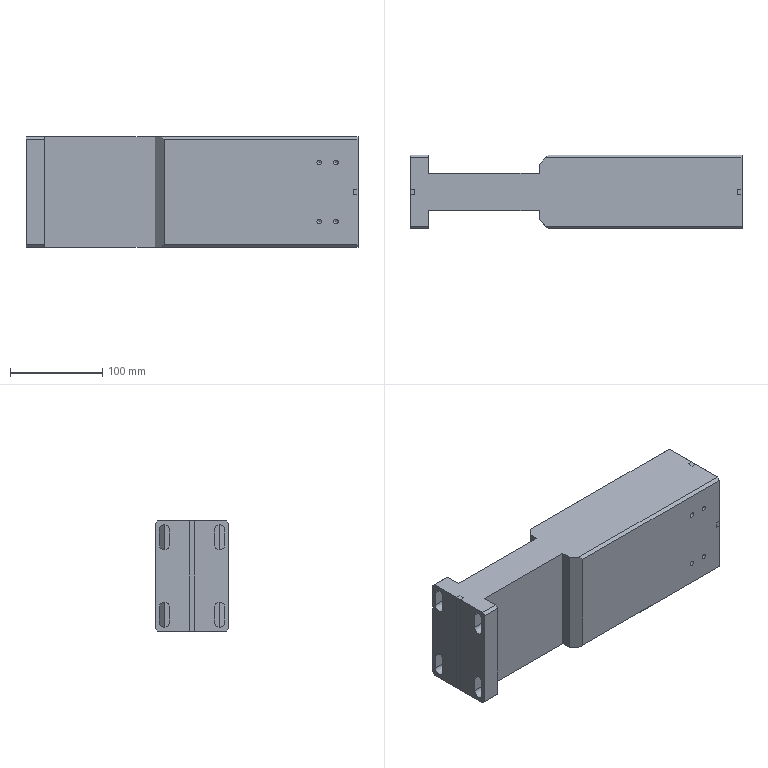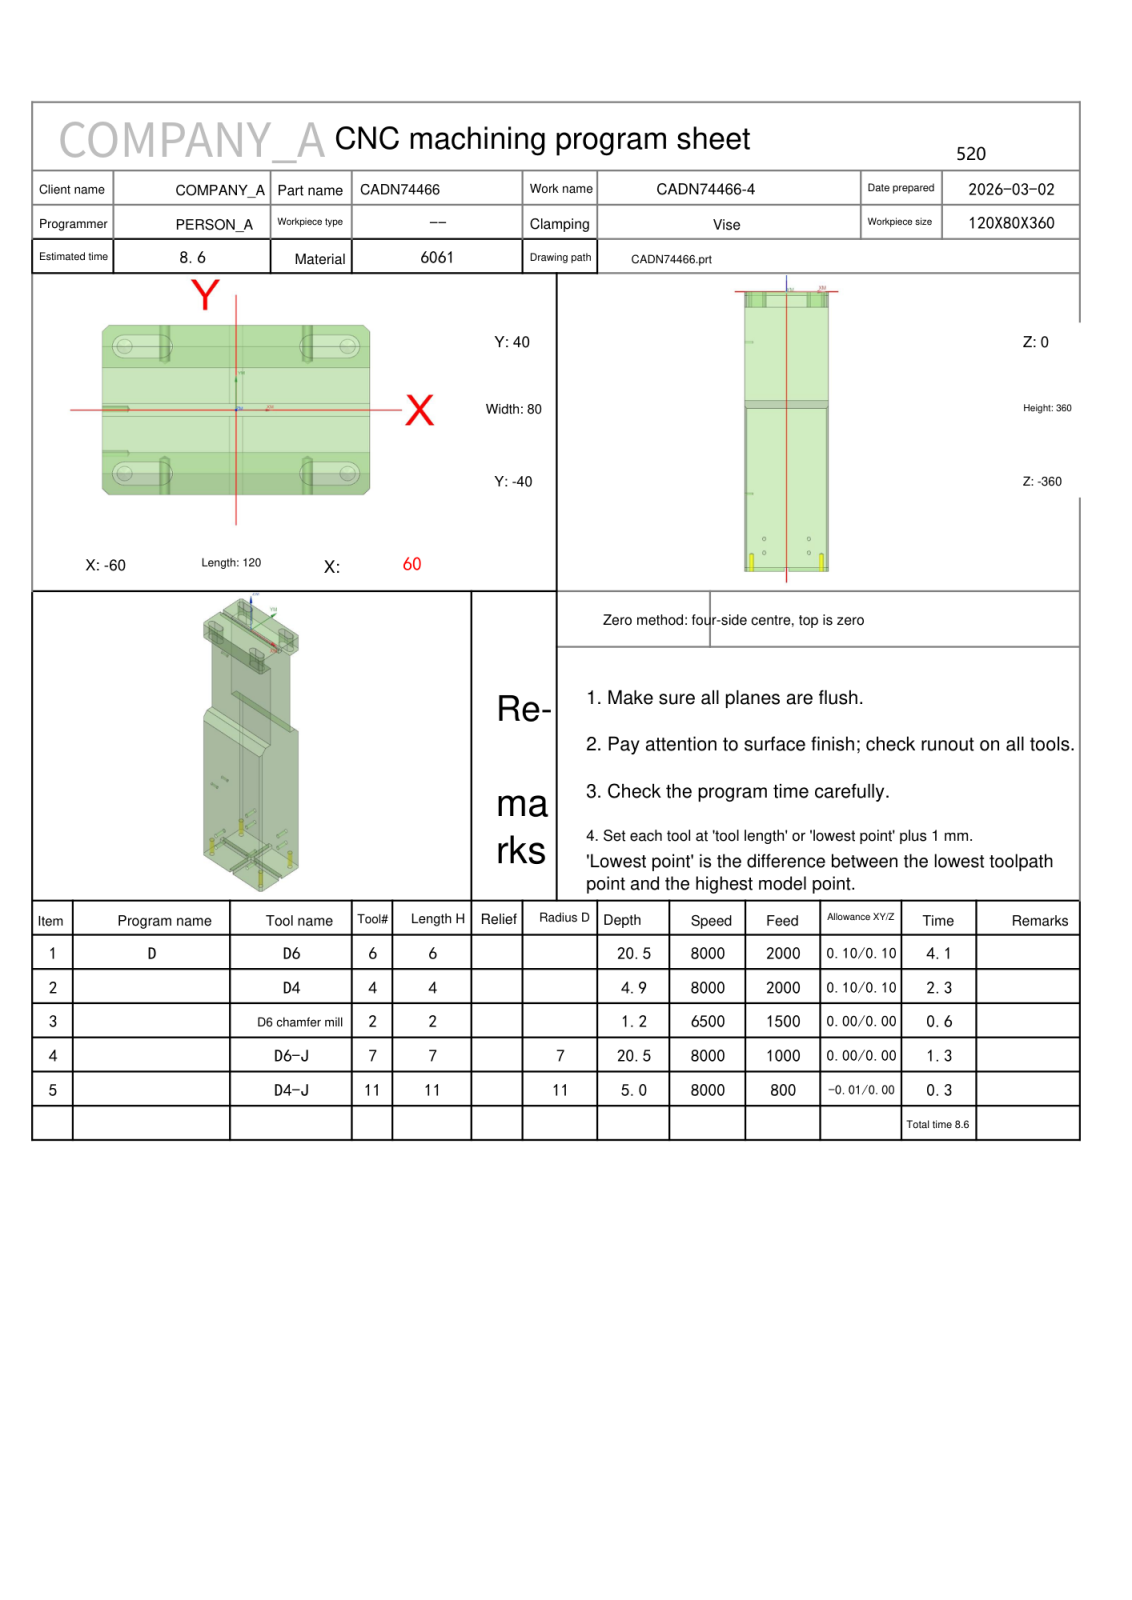NC program | NX | posted by the shop | part box 360 x 80 x 120 mm
Whole program, first 1424 of 1794 lines:
%
O0001
(Machine time: 9.60 MIN)
(===Total Tool:5===)
(T6=D6      D=6.   R=0.   D-  H06 Z=-20.5 )
(T4=D4      D=4.   R=0.   D-  H04 Z=-4.9  )
(T2=D6 chamfer mill   D=6.   R=0.   D-  H02 Z=-1.2  )
(T7=D6-J    D=6.   R=0.   D7  H07 Z=-20.5 )
(T11=D4-J   D=4.   R=0.   D11 H11 Z=-5.   )
G80 G90 G17 G49 G40
G91 G28 Z0
M01
N1 T06 M06
(D6  D=6. R=0. H=06 ce=0.10 di=0.10)
G00 G90 G54 X-38.502 Y-27.6 M03 S8000
G43 H06 Z50.
M08
Z1.
G01 X-50.381 Z.377 F2000.
X-51.324 Y-27.962 Z.325
X-52.038 Y-28.676 Z.272
X-52.4 Y-29.619 Z.219
Y-30.381 Z.179
X-52.038 Y-31.324 Z.126
X-51.324 Y-32.038 Z.073
X-50.381 Y-32.4 Z.02
X-50. Z0.0
X-34. Z-.166
G03 X-31.6 Y-30. Z-.205 I0.0 J2.4
X-34. Y-27.6 Z-.244 I-2.4 J0.0
G01 X-50. Z-.41
G03 X-52.4 Y-30. Z-.449 I0.0 J-2.4
X-50. Y-32.4 Z-.488 I2.4 J0.0
G01 X-34. Z-.654
G03 X-31.6 Y-30. Z-.693 I0.0 J2.4
X-34. Y-27.6 Z-.732 I-2.4 J0.0
G01 X-50. Z-.898
G03 X-52.4 Y-30. Z-.937 I0.0 J-2.4
X-50. Y-32.4 Z-.976 I2.4 J0.0
G01 X-34. Z-1.142
G03 X-31.6 Y-30. Z-1.181 I0.0 J2.4
X-34. Y-27.6 Z-1.22 I-2.4 J0.0
G01 X-50. Z-1.386
G03 X-52.4 Y-30. Z-1.425 I0.0 J-2.4
X-50. Y-32.4 Z-1.464 I2.4 J0.0
G01 X-34. Z-1.63
G03 X-31.6 Y-30. Z-1.669 I0.0 J2.4
X-34. Y-27.6 Z-1.708 I-2.4 J0.0
G01 X-50. Z-1.874
G03 X-52.4 Y-30. Z-1.913 I0.0 J-2.4
X-50. Y-32.4 Z-1.952 I2.4 J0.0
G01 X-34. Z-2.118
G03 X-31.6 Y-30. Z-2.157 I0.0 J2.4
X-34. Y-27.6 Z-2.196 I-2.4 J0.0
G01 X-50. Z-2.362
G03 X-52.4 Y-30. Z-2.401 I0.0 J-2.4
X-50. Y-32.4 Z-2.44 I2.4 J0.0
G01 X-34. Z-2.606
G03 X-31.6 Y-30. Z-2.645 I0.0 J2.4
X-34. Y-27.6 Z-2.685 I-2.4 J0.0
G01 X-50. Z-2.85
G03 X-52.4 Y-30. Z-2.889 I0.0 J-2.4
X-50. Y-32.4 Z-2.929 I2.4 J0.0
G01 X-34. Z-3.094
G03 X-31.6 Y-30. Z-3.134 I0.0 J2.4
X-34. Y-27.6 Z-3.173 I-2.4 J0.0
G01 X-50. Z-3.338
G03 X-52.4 Y-30. Z-3.378 I0.0 J-2.4
X-50. Y-32.4 Z-3.417 I2.4 J0.0
G01 X-34. Z-3.583
G03 X-31.6 Y-30. Z-3.622 I0.0 J2.4
X-34. Y-27.6 Z-3.661 I-2.4 J0.0
G01 X-50. Z-3.827
G03 X-52.4 Y-30. Z-3.866 I0.0 J-2.4
X-50. Y-32.4 Z-3.905 I2.4 J0.0
G01 X-34. Z-4.071
G03 X-31.6 Y-30. Z-4.11 I0.0 J2.4
X-34. Y-27.6 Z-4.149 I-2.4 J0.0
G01 X-50. Z-4.315
G03 X-52.4 Y-30. Z-4.354 I0.0 J-2.4
X-50. Y-32.4 Z-4.393 I2.4 J0.0
G01 X-34. Z-4.559
G03 X-31.6 Y-30. Z-4.598 I0.0 J2.4
X-34. Y-27.6 Z-4.637 I-2.4 J0.0
G01 X-50. Z-4.803
G03 X-52.4 Y-30. Z-4.842 I0.0 J-2.4
X-50. Y-32.4 Z-4.881 I2.4 J0.0
G01 X-34. Z-5.047
G03 X-31.6 Y-30. Z-5.086 I0.0 J2.4
X-34. Y-27.6 Z-5.125 I-2.4 J0.0
G01 X-50. Z-5.291
G03 X-52.4 Y-30. Z-5.33 I0.0 J-2.4
X-50. Y-32.4 Z-5.369 I2.4 J0.0
G01 X-34. Z-5.535
G03 X-31.6 Y-30. Z-5.574 I0.0 J2.4
X-34. Y-27.6 Z-5.613 I-2.4 J0.0
G01 X-50. Z-5.779
G03 X-52.4 Y-30. Z-5.818 I0.0 J-2.4
X-50. Y-32.4 Z-5.857 I2.4 J0.0
G01 X-34. Z-6.023
G03 X-31.6 Y-30. Z-6.062 I0.0 J2.4
X-34. Y-27.6 Z-6.101 I-2.4 J0.0
G01 X-50. Z-6.267
G03 X-52.4 Y-30. Z-6.306 I0.0 J-2.4
X-50. Y-32.4 Z-6.345 I2.4 J0.0
G01 X-34. Z-6.511
G03 X-31.6 Y-30. Z-6.55 I0.0 J2.4
X-34. Y-27.6 Z-6.589 I-2.4 J0.0
G01 X-50. Z-6.755
G03 X-52.4 Y-30. Z-6.794 I0.0 J-2.4
X-50. Y-32.4 Z-6.833 I2.4 J0.0
G01 X-34. Z-6.999
G03 X-31.6 Y-30. Z-7.038 I0.0 J2.4
X-34. Y-27.6 Z-7.077 I-2.4 J0.0
G01 X-50. Z-7.243
G03 X-52.4 Y-30. Z-7.282 I0.0 J-2.4
X-50. Y-32.4 Z-7.321 I2.4 J0.0
G01 X-34. Z-7.487
G03 X-31.6 Y-30. Z-7.526 I0.0 J2.4
X-34. Y-27.6 Z-7.565 I-2.4 J0.0
G01 X-50. Z-7.731
G03 X-52.4 Y-30. Z-7.77 I0.0 J-2.4
X-50. Y-32.4 Z-7.81 I2.4 J0.0
G01 X-34. Z-7.975
G03 X-31.6 Y-30. Z-8.014 I0.0 J2.4
X-34. Y-27.6 Z-8.054 I-2.4 J0.0
G01 X-50. Z-8.219
G03 X-52.4 Y-30. Z-8.259 I0.0 J-2.4
X-50. Y-32.4 Z-8.298 I2.4 J0.0
G01 X-34. Z-8.463
G03 X-31.6 Y-30. Z-8.503 I0.0 J2.4
X-34. Y-27.6 Z-8.542 I-2.4 J0.0
G01 X-50. Z-8.708
G03 X-52.4 Y-30. Z-8.747 I0.0 J-2.4
X-50. Y-32.4 Z-8.786 I2.4 J0.0
G01 X-34. Z-8.952
G03 X-31.6 Y-30. Z-8.991 I0.0 J2.4
X-34. Y-27.6 Z-9.03 I-2.4 J0.0
G01 X-50. Z-9.196
G03 X-52.4 Y-30. Z-9.235 I0.0 J-2.4
X-50. Y-32.4 Z-9.274 I2.4 J0.0
G01 X-34. Z-9.44
G03 X-31.6 Y-30. Z-9.479 I0.0 J2.4
X-34. Y-27.6 Z-9.518 I-2.4 J0.0
G01 X-50. Z-9.684
G03 X-52.4 Y-30. Z-9.723 I0.0 J-2.4
X-50. Y-32.4 Z-9.762 I2.4 J0.0
G01 X-34. Z-9.928
G03 X-31.6 Y-30. Z-9.967 I0.0 J2.4
X-34. Y-27.6 Z-10.006 I-2.4 J0.0
G01 X-50. Z-10.172
G03 X-52.4 Y-30. Z-10.211 I0.0 J-2.4
X-50. Y-32.4 Z-10.25 I2.4 J0.0
G01 X-34. Z-10.416
G03 X-31.6 Y-30. Z-10.455 I0.0 J2.4
X-34. Y-27.6 Z-10.494 I-2.4 J0.0
G01 X-50. Z-10.66
G03 X-52.4 Y-30. Z-10.699 I0.0 J-2.4
X-50. Y-32.4 Z-10.738 I2.4 J0.0
G01 X-34. Z-10.904
G03 X-31.6 Y-30. Z-10.943 I0.0 J2.4
X-34. Y-27.6 Z-10.982 I-2.4 J0.0
G01 X-50. Z-11.148
G03 X-52.4 Y-30. Z-11.187 I0.0 J-2.4
X-50. Y-32.4 Z-11.226 I2.4 J0.0
G01 X-34. Z-11.392
G03 X-31.6 Y-30. Z-11.431 I0.0 J2.4
X-34. Y-27.6 Z-11.47 I-2.4 J0.0
G01 X-50. Z-11.636
G03 X-52.4 Y-30. Z-11.675 I0.0 J-2.4
X-50. Y-32.4 Z-11.714 I2.4 J0.0
G01 X-34. Z-11.88
G03 X-31.6 Y-30. Z-11.919 I0.0 J2.4
X-34. Y-27.6 Z-11.958 I-2.4 J0.0
G01 X-50. Z-12.124
G03 X-52.4 Y-30. Z-12.163 I0.0 J-2.4
X-50. Y-32.4 Z-12.202 I2.4 J0.0
G01 X-34. Z-12.368
G03 X-31.6 Y-30. Z-12.407 I0.0 J2.4
X-34. Y-27.6 Z-12.446 I-2.4 J0.0
G01 X-50. Z-12.612
G03 X-52.4 Y-30. Z-12.651 I0.0 J-2.4
X-50. Y-32.4 Z-12.69 I2.4 J0.0
G01 X-34. Z-12.856
G03 X-31.6 Y-30. Z-12.895 I0.0 J2.4
X-34. Y-27.6 Z-12.935 I-2.4 J0.0
G01 X-50. Z-13.1
G03 X-52.4 Y-30. Z-13.139 I0.0 J-2.4
X-50. Y-32.4 Z-13.179 I2.4 J0.0
G01 X-34. Z-13.344
G03 X-31.6 Y-30. Z-13.384 I0.0 J2.4
X-34. Y-27.6 Z-13.423 I-2.4 J0.0
G01 X-50. Z-13.588
G03 X-52.4 Y-30. Z-13.628 I0.0 J-2.4
X-50. Y-32.4 Z-13.667 I2.4 J0.0
G01 X-34. Z-13.833
G03 X-31.6 Y-30. Z-13.872 I0.0 J2.4
X-34. Y-27.6 Z-13.911 I-2.4 J0.0
G01 X-50. Z-14.077
G03 X-52.4 Y-30. Z-14.116 I0.0 J-2.4
X-50. Y-32.4 Z-14.155 I2.4 J0.0
G01 X-34. Z-14.321
G03 X-31.6 Y-30. Z-14.36 I0.0 J2.4
X-34. Y-27.6 Z-14.399 I-2.4 J0.0
G01 X-50. Z-14.565
G03 X-52.4 Y-30. Z-14.604 I0.0 J-2.4
X-50. Y-32.4 Z-14.643 I2.4 J0.0
G01 X-34. Z-14.809
G03 X-31.6 Y-30. Z-14.848 I0.0 J2.4
X-34. Y-27.6 Z-14.887 I-2.4 J0.0
G01 X-50. Z-15.053
G03 X-52.4 Y-30. Z-15.092 I0.0 J-2.4
X-50. Y-32.4 Z-15.131 I2.4 J0.0
G01 X-34. Z-15.297
G03 X-31.6 Y-30. Z-15.336 I0.0 J2.4
X-34. Y-27.6 Z-15.375 I-2.4 J0.0
G01 X-50. Z-15.541
G03 X-52.4 Y-30. Z-15.58 I0.0 J-2.4
X-50. Y-32.4 Z-15.619 I2.4 J0.0
G01 X-34. Z-15.785
G03 X-31.6 Y-30. Z-15.824 I0.0 J2.4
X-34. Y-27.6 Z-15.863 I-2.4 J0.0
G01 X-50. Z-16.029
G03 X-52.4 Y-30. Z-16.068 I0.0 J-2.4
X-50. Y-32.4 Z-16.107 I2.4 J0.0
G01 X-34. Z-16.273
G03 X-31.6 Y-30. Z-16.312 I0.0 J2.4
X-34. Y-27.6 Z-16.351 I-2.4 J0.0
G01 X-50. Z-16.517
G03 X-52.4 Y-30. Z-16.556 I0.0 J-2.4
X-50. Y-32.4 Z-16.595 I2.4 J0.0
G01 X-34. Z-16.761
G03 X-31.6 Y-30. Z-16.8 I0.0 J2.4
X-34. Y-27.6 Z-16.839 I-2.4 J0.0
G01 X-50. Z-17.005
G03 X-52.4 Y-30. Z-17.044 I0.0 J-2.4
X-50. Y-32.4 Z-17.083 I2.4 J0.0
G01 X-34. Z-17.249
G03 X-31.6 Y-30. Z-17.288 I0.0 J2.4
X-34. Y-27.6 Z-17.327 I-2.4 J0.0
G01 X-50. Z-17.493
G03 X-52.4 Y-30. Z-17.532 I0.0 J-2.4
X-50. Y-32.4 Z-17.571 I2.4 J0.0
G01 X-34. Z-17.737
G03 X-31.6 Y-30. Z-17.776 I0.0 J2.4
X-34. Y-27.6 Z-17.815 I-2.4 J0.0
G01 X-50. Z-17.981
G03 X-52.4 Y-30. Z-18.02 I0.0 J-2.4
X-50. Y-32.4 Z-18.06 I2.4 J0.0
G01 X-34. Z-18.225
G03 X-31.6 Y-30. Z-18.264 I0.0 J2.4
X-34. Y-27.6 Z-18.304 I-2.4 J0.0
G01 X-50. Z-18.469
G03 X-52.4 Y-30. Z-18.509 I0.0 J-2.4
X-50. Y-32.4 Z-18.548 I2.4 J0.0
G01 X-34. Z-18.713
G03 X-31.6 Y-30. Z-18.753 I0.0 J2.4
X-34. Y-27.6 Z-18.792 I-2.4 J0.0
G01 X-50. Z-18.958
G03 X-52.4 Y-30. Z-18.997 I0.0 J-2.4
X-50. Y-32.4 Z-19.036 I2.4 J0.0
G01 X-34. Z-19.202
G03 X-31.6 Y-30. Z-19.241 I0.0 J2.4
X-34. Y-27.6 Z-19.28 I-2.4 J0.0
G01 X-50. Z-19.446
G03 X-52.4 Y-30. Z-19.485 I0.0 J-2.4
X-50. Y-32.4 Z-19.524 I2.4 J0.0
G01 X-34. Z-19.69
G03 X-31.6 Y-30. Z-19.729 I0.0 J2.4
X-34. Y-27.6 Z-19.768 I-2.4 J0.0
G01 X-50. Z-19.934
G03 X-52.4 Y-30. Z-19.973 I0.0 J-2.4
X-50. Y-32.4 Z-20.012 I2.4 J0.0
G01 X-34. Z-20.178
G03 X-31.6 Y-30. Z-20.217 I0.0 J2.4
X-34. Y-27.6 Z-20.256 I-2.4 J0.0
G01 X-50. Z-20.422
G03 X-52.4 Y-30. Z-20.461 I0.0 J-2.4
X-50. Y-32.4 Z-20.5 I2.4 J0.0
G01 X-34.
G03 X-31.6 Y-30. I0.0 J2.4
X-34. Y-27.6 I-2.4 J0.0
G01 X-50.
G03 X-52.4 Y-30. I0.0 J-2.4
X-50. Y-32.4 I2.4 J0.0
G01 X-49.6
Z-19.5
G00 Z50.
X-45.498 Y27.6
Z1.
G01 X-33.619 Z.377
X-32.676 Y27.962 Z.325
X-31.962 Y28.676 Z.272
X-31.6 Y29.619 Z.219
Y30.381 Z.179
X-31.962 Y31.324 Z.126
X-32.676 Y32.038 Z.073
X-33.619 Y32.4 Z.02
X-34. Z0.0
X-50. Z-.166
G03 X-52.4 Y30. Z-.205 I0.0 J-2.4
X-50. Y27.6 Z-.244 I2.4 J0.0
G01 X-34. Z-.41
G03 X-31.6 Y30. Z-.449 I0.0 J2.4
X-34. Y32.4 Z-.488 I-2.4 J0.0
G01 X-50. Z-.654
G03 X-52.4 Y30. Z-.693 I0.0 J-2.4
X-50. Y27.6 Z-.732 I2.4 J0.0
G01 X-34. Z-.898
G03 X-31.6 Y30. Z-.937 I0.0 J2.4
X-34. Y32.4 Z-.976 I-2.4 J0.0
G01 X-50. Z-1.142
G03 X-52.4 Y30. Z-1.181 I0.0 J-2.4
X-50. Y27.6 Z-1.22 I2.4 J0.0
G01 X-34. Z-1.386
G03 X-31.6 Y30. Z-1.425 I0.0 J2.4
X-34. Y32.4 Z-1.464 I-2.4 J0.0
G01 X-50. Z-1.63
G03 X-52.4 Y30. Z-1.669 I0.0 J-2.4
X-50. Y27.6 Z-1.708 I2.4 J0.0
G01 X-34. Z-1.874
G03 X-31.6 Y30. Z-1.913 I0.0 J2.4
X-34. Y32.4 Z-1.952 I-2.4 J0.0
G01 X-50. Z-2.118
G03 X-52.4 Y30. Z-2.157 I0.0 J-2.4
X-50. Y27.6 Z-2.196 I2.4 J0.0
G01 X-34. Z-2.362
G03 X-31.6 Y30. Z-2.401 I0.0 J2.4
X-34. Y32.4 Z-2.44 I-2.4 J0.0
G01 X-50. Z-2.606
G03 X-52.4 Y30. Z-2.645 I0.0 J-2.4
X-50. Y27.6 Z-2.685 I2.4 J0.0
G01 X-34. Z-2.85
G03 X-31.6 Y30. Z-2.889 I0.0 J2.4
X-34. Y32.4 Z-2.929 I-2.4 J0.0
G01 X-50. Z-3.094
G03 X-52.4 Y30. Z-3.134 I0.0 J-2.4
X-50. Y27.6 Z-3.173 I2.4 J0.0
G01 X-34. Z-3.338
G03 X-31.6 Y30. Z-3.378 I0.0 J2.4
X-34. Y32.4 Z-3.417 I-2.4 J0.0
G01 X-50. Z-3.583
G03 X-52.4 Y30. Z-3.622 I0.0 J-2.4
X-50. Y27.6 Z-3.661 I2.4 J0.0
G01 X-34. Z-3.827
G03 X-31.6 Y30. Z-3.866 I0.0 J2.4
X-34. Y32.4 Z-3.905 I-2.4 J0.0
G01 X-50. Z-4.071
G03 X-52.4 Y30. Z-4.11 I0.0 J-2.4
X-50. Y27.6 Z-4.149 I2.4 J0.0
G01 X-34. Z-4.315
G03 X-31.6 Y30. Z-4.354 I0.0 J2.4
X-34. Y32.4 Z-4.393 I-2.4 J0.0
G01 X-50. Z-4.559
G03 X-52.4 Y30. Z-4.598 I0.0 J-2.4
X-50. Y27.6 Z-4.637 I2.4 J0.0
G01 X-34. Z-4.803
G03 X-31.6 Y30. Z-4.842 I0.0 J2.4
X-34. Y32.4 Z-4.881 I-2.4 J0.0
G01 X-50. Z-5.047
G03 X-52.4 Y30. Z-5.086 I0.0 J-2.4
X-50. Y27.6 Z-5.125 I2.4 J0.0
G01 X-34. Z-5.291
G03 X-31.6 Y30. Z-5.33 I0.0 J2.4
X-34. Y32.4 Z-5.369 I-2.4 J0.0
G01 X-50. Z-5.535
G03 X-52.4 Y30. Z-5.574 I0.0 J-2.4
X-50. Y27.6 Z-5.613 I2.4 J0.0
G01 X-34. Z-5.779
G03 X-31.6 Y30. Z-5.818 I0.0 J2.4
X-34. Y32.4 Z-5.857 I-2.4 J0.0
G01 X-50. Z-6.023
G03 X-52.4 Y30. Z-6.062 I0.0 J-2.4
X-50. Y27.6 Z-6.101 I2.4 J0.0
G01 X-34. Z-6.267
G03 X-31.6 Y30. Z-6.306 I0.0 J2.4
X-34. Y32.4 Z-6.345 I-2.4 J0.0
G01 X-50. Z-6.511
G03 X-52.4 Y30. Z-6.55 I0.0 J-2.4
X-50. Y27.6 Z-6.589 I2.4 J0.0
G01 X-34. Z-6.755
G03 X-31.6 Y30. Z-6.794 I0.0 J2.4
X-34. Y32.4 Z-6.833 I-2.4 J0.0
G01 X-50. Z-6.999
G03 X-52.4 Y30. Z-7.038 I0.0 J-2.4
X-50. Y27.6 Z-7.077 I2.4 J0.0
G01 X-34. Z-7.243
G03 X-31.6 Y30. Z-7.282 I0.0 J2.4
X-34. Y32.4 Z-7.321 I-2.4 J0.0
G01 X-50. Z-7.487
G03 X-52.4 Y30. Z-7.526 I0.0 J-2.4
X-50. Y27.6 Z-7.565 I2.4 J0.0
G01 X-34. Z-7.731
G03 X-31.6 Y30. Z-7.77 I0.0 J2.4
X-34. Y32.4 Z-7.81 I-2.4 J0.0
G01 X-50. Z-7.975
G03 X-52.4 Y30. Z-8.014 I0.0 J-2.4
X-50. Y27.6 Z-8.054 I2.4 J0.0
G01 X-34. Z-8.219
G03 X-31.6 Y30. Z-8.259 I0.0 J2.4
X-34. Y32.4 Z-8.298 I-2.4 J0.0
G01 X-50. Z-8.463
G03 X-52.4 Y30. Z-8.503 I0.0 J-2.4
X-50. Y27.6 Z-8.542 I2.4 J0.0
G01 X-34. Z-8.708
G03 X-31.6 Y30. Z-8.747 I0.0 J2.4
X-34. Y32.4 Z-8.786 I-2.4 J0.0
G01 X-50. Z-8.952
G03 X-52.4 Y30. Z-8.991 I0.0 J-2.4
X-50. Y27.6 Z-9.03 I2.4 J0.0
G01 X-34. Z-9.196
G03 X-31.6 Y30. Z-9.235 I0.0 J2.4
X-34. Y32.4 Z-9.274 I-2.4 J0.0
G01 X-50. Z-9.44
G03 X-52.4 Y30. Z-9.479 I0.0 J-2.4
X-50. Y27.6 Z-9.518 I2.4 J0.0
G01 X-34. Z-9.684
G03 X-31.6 Y30. Z-9.723 I0.0 J2.4
X-34. Y32.4 Z-9.762 I-2.4 J0.0
G01 X-50. Z-9.928
G03 X-52.4 Y30. Z-9.967 I0.0 J-2.4
X-50. Y27.6 Z-10.006 I2.4 J0.0
G01 X-34. Z-10.172
G03 X-31.6 Y30. Z-10.211 I0.0 J2.4
X-34. Y32.4 Z-10.25 I-2.4 J0.0
G01 X-50. Z-10.416
G03 X-52.4 Y30. Z-10.455 I0.0 J-2.4
X-50. Y27.6 Z-10.494 I2.4 J0.0
G01 X-34. Z-10.66
G03 X-31.6 Y30. Z-10.699 I0.0 J2.4
X-34. Y32.4 Z-10.738 I-2.4 J0.0
G01 X-50. Z-10.904
G03 X-52.4 Y30. Z-10.943 I0.0 J-2.4
X-50. Y27.6 Z-10.982 I2.4 J0.0
G01 X-34. Z-11.148
G03 X-31.6 Y30. Z-11.187 I0.0 J2.4
X-34. Y32.4 Z-11.226 I-2.4 J0.0
G01 X-50. Z-11.392
G03 X-52.4 Y30. Z-11.431 I0.0 J-2.4
X-50. Y27.6 Z-11.47 I2.4 J0.0
G01 X-34. Z-11.636
G03 X-31.6 Y30. Z-11.675 I0.0 J2.4
X-34. Y32.4 Z-11.714 I-2.4 J0.0
G01 X-50. Z-11.88
G03 X-52.4 Y30. Z-11.919 I0.0 J-2.4
X-50. Y27.6 Z-11.958 I2.4 J0.0
G01 X-34. Z-12.124
G03 X-31.6 Y30. Z-12.163 I0.0 J2.4
X-34. Y32.4 Z-12.202 I-2.4 J0.0
G01 X-50. Z-12.368
G03 X-52.4 Y30. Z-12.407 I0.0 J-2.4
X-50. Y27.6 Z-12.446 I2.4 J0.0
G01 X-34. Z-12.612
G03 X-31.6 Y30. Z-12.651 I0.0 J2.4
X-34. Y32.4 Z-12.69 I-2.4 J0.0
G01 X-50. Z-12.856
G03 X-52.4 Y30. Z-12.895 I0.0 J-2.4
X-50. Y27.6 Z-12.935 I2.4 J0.0
G01 X-34. Z-13.1
G03 X-31.6 Y30. Z-13.139 I0.0 J2.4
X-34. Y32.4 Z-13.179 I-2.4 J0.0
G01 X-50. Z-13.344
G03 X-52.4 Y30. Z-13.384 I0.0 J-2.4
X-50. Y27.6 Z-13.423 I2.4 J0.0
G01 X-34. Z-13.588
G03 X-31.6 Y30. Z-13.628 I0.0 J2.4
X-34. Y32.4 Z-13.667 I-2.4 J0.0
G01 X-50. Z-13.833
G03 X-52.4 Y30. Z-13.872 I0.0 J-2.4
X-50. Y27.6 Z-13.911 I2.4 J0.0
G01 X-34. Z-14.077
G03 X-31.6 Y30. Z-14.116 I0.0 J2.4
X-34. Y32.4 Z-14.155 I-2.4 J0.0
G01 X-50. Z-14.321
G03 X-52.4 Y30. Z-14.36 I0.0 J-2.4
X-50. Y27.6 Z-14.399 I2.4 J0.0
G01 X-34. Z-14.565
G03 X-31.6 Y30. Z-14.604 I0.0 J2.4
X-34. Y32.4 Z-14.643 I-2.4 J0.0
G01 X-50. Z-14.809
G03 X-52.4 Y30. Z-14.848 I0.0 J-2.4
X-50. Y27.6 Z-14.887 I2.4 J0.0
G01 X-34. Z-15.053
G03 X-31.6 Y30. Z-15.092 I0.0 J2.4
X-34. Y32.4 Z-15.131 I-2.4 J0.0
G01 X-50. Z-15.297
G03 X-52.4 Y30. Z-15.336 I0.0 J-2.4
X-50. Y27.6 Z-15.375 I2.4 J0.0
G01 X-34. Z-15.541
G03 X-31.6 Y30. Z-15.58 I0.0 J2.4
X-34. Y32.4 Z-15.619 I-2.4 J0.0
G01 X-50. Z-15.785
G03 X-52.4 Y30. Z-15.824 I0.0 J-2.4
X-50. Y27.6 Z-15.863 I2.4 J0.0
G01 X-34. Z-16.029
G03 X-31.6 Y30. Z-16.068 I0.0 J2.4
X-34. Y32.4 Z-16.107 I-2.4 J0.0
G01 X-50. Z-16.273
G03 X-52.4 Y30. Z-16.312 I0.0 J-2.4
X-50. Y27.6 Z-16.351 I2.4 J0.0
G01 X-34. Z-16.517
G03 X-31.6 Y30. Z-16.556 I0.0 J2.4
X-34. Y32.4 Z-16.595 I-2.4 J0.0
G01 X-50. Z-16.761
G03 X-52.4 Y30. Z-16.8 I0.0 J-2.4
X-50. Y27.6 Z-16.839 I2.4 J0.0
G01 X-34. Z-17.005
G03 X-31.6 Y30. Z-17.044 I0.0 J2.4
X-34. Y32.4 Z-17.083 I-2.4 J0.0
G01 X-50. Z-17.249
G03 X-52.4 Y30. Z-17.288 I0.0 J-2.4
X-50. Y27.6 Z-17.327 I2.4 J0.0
G01 X-34. Z-17.493
G03 X-31.6 Y30. Z-17.532 I0.0 J2.4
X-34. Y32.4 Z-17.571 I-2.4 J0.0
G01 X-50. Z-17.737
G03 X-52.4 Y30. Z-17.776 I0.0 J-2.4
X-50. Y27.6 Z-17.815 I2.4 J0.0
G01 X-34. Z-17.981
G03 X-31.6 Y30. Z-18.02 I0.0 J2.4
X-34. Y32.4 Z-18.06 I-2.4 J0.0
G01 X-50. Z-18.225
G03 X-52.4 Y30. Z-18.264 I0.0 J-2.4
X-50. Y27.6 Z-18.304 I2.4 J0.0
G01 X-34. Z-18.469
G03 X-31.6 Y30. Z-18.509 I0.0 J2.4
X-34. Y32.4 Z-18.548 I-2.4 J0.0
G01 X-50. Z-18.713
G03 X-52.4 Y30. Z-18.753 I0.0 J-2.4
X-50. Y27.6 Z-18.792 I2.4 J0.0
G01 X-34. Z-18.958
G03 X-31.6 Y30. Z-18.997 I0.0 J2.4
X-34. Y32.4 Z-19.036 I-2.4 J0.0
G01 X-50. Z-19.202
G03 X-52.4 Y30. Z-19.241 I0.0 J-2.4
X-50. Y27.6 Z-19.28 I2.4 J0.0
G01 X-34. Z-19.446
G03 X-31.6 Y30. Z-19.485 I0.0 J2.4
X-34. Y32.4 Z-19.524 I-2.4 J0.0
G01 X-50. Z-19.69
G03 X-52.4 Y30. Z-19.729 I0.0 J-2.4
X-50. Y27.6 Z-19.768 I2.4 J0.0
G01 X-34. Z-19.934
G03 X-31.6 Y30. Z-19.973 I0.0 J2.4
X-34. Y32.4 Z-20.012 I-2.4 J0.0
G01 X-50. Z-20.178
G03 X-52.4 Y30. Z-20.217 I0.0 J-2.4
X-50. Y27.6 Z-20.256 I2.4 J0.0
G01 X-34. Z-20.422
G03 X-31.6 Y30. Z-20.461 I0.0 J2.4
X-34. Y32.4 Z-20.5 I-2.4 J0.0
G01 X-50.
G03 X-52.4 Y30. I0.0 J-2.4
X-50. Y27.6 I2.4 J0.0
G01 X-34.
G03 X-31.6 Y30. I0.0 J2.4
X-34. Y32.4 I-2.4 J0.0
G01 X-34.4
Z-19.5
G00 Z50.
X38.502 Y27.6
Z1.
G01 X50.381 Z.377
X51.324 Y27.962 Z.325
X52.038 Y28.676 Z.272
X52.4 Y29.619 Z.219
Y30.381 Z.179
X52.038 Y31.324 Z.126
X51.324 Y32.038 Z.073
X50.381 Y32.4 Z.02
X50. Z0.0
X34. Z-.17
G03 X31.6 Y30. Z-.21 I0.0 J-2.4
X34. Y27.6 Z-.25 I2.4 J0.0
G01 X50. Z-.42
G03 X52.4 Y30. Z-.46 I0.0 J2.4
X50. Y32.4 Z-.5 I-2.4 J0.0
G01 X34. Z-.67
G03 X31.6 Y30. Z-.71 I0.0 J-2.4
X34. Y27.6 Z-.75 I2.4 J0.0
G01 X50. Z-.92
G03 X52.4 Y30. Z-.96 I0.0 J2.4
X50. Y32.4 Z-1. I-2.4 J0.0
G01 X34. Z-1.17
G03 X31.6 Y30. Z-1.21 I0.0 J-2.4
X34. Y27.6 Z-1.25 I2.4 J0.0
G01 X50. Z-1.42
G03 X52.4 Y30. Z-1.46 I0.0 J2.4
X50. Y32.4 Z-1.5 I-2.4 J0.0
G01 X34. Z-1.67
G03 X31.6 Y30. Z-1.71 I0.0 J-2.4
X34. Y27.6 Z-1.75 I2.4 J0.0
G01 X50. Z-1.92
G03 X52.4 Y30. Z-1.96 I0.0 J2.4
X50. Y32.4 Z-2. I-2.4 J0.0
G01 X34. Z-2.17
G03 X31.6 Y30. Z-2.21 I0.0 J-2.4
X34. Y27.6 Z-2.25 I2.4 J0.0
G01 X50. Z-2.42
G03 X52.4 Y30. Z-2.46 I0.0 J2.4
X50. Y32.4 Z-2.5 I-2.4 J0.0
G01 X34. Z-2.67
G03 X31.6 Y30. Z-2.71 I0.0 J-2.4
X34. Y27.6 Z-2.75 I2.4 J0.0
G01 X50. Z-2.92
G03 X52.4 Y30. Z-2.96 I0.0 J2.4
X50. Y32.4 Z-3. I-2.4 J0.0
G01 X34. Z-3.17
G03 X31.6 Y30. Z-3.21 I0.0 J-2.4
X34. Y27.6 Z-3.25 I2.4 J0.0
G01 X50. Z-3.42
G03 X52.4 Y30. Z-3.46 I0.0 J2.4
X50. Y32.4 Z-3.5 I-2.4 J0.0
G01 X34. Z-3.67
G03 X31.6 Y30. Z-3.71 I0.0 J-2.4
X34. Y27.6 Z-3.75 I2.4 J0.0
G01 X50. Z-3.92
G03 X52.4 Y30. Z-3.96 I0.0 J2.4
X50. Y32.4 Z-4. I-2.4 J0.0
G01 X34. Z-4.17
G03 X31.6 Y30. Z-4.21 I0.0 J-2.4
X34. Y27.6 Z-4.25 I2.4 J0.0
G01 X50. Z-4.42
G03 X52.4 Y30. Z-4.46 I0.0 J2.4
X50. Y32.4 Z-4.5 I-2.4 J0.0
G01 X34. Z-4.67
G03 X31.6 Y30. Z-4.71 I0.0 J-2.4
X34. Y27.6 Z-4.75 I2.4 J0.0
G01 X50. Z-4.92
G03 X52.4 Y30. Z-4.96 I0.0 J2.4
X50. Y32.4 Z-5. I-2.4 J0.0
G01 X34. Z-5.17
G03 X31.6 Y30. Z-5.21 I0.0 J-2.4
X34. Y27.6 Z-5.25 I2.4 J0.0
G01 X50. Z-5.42
G03 X52.4 Y30. Z-5.46 I0.0 J2.4
X50. Y32.4 Z-5.5 I-2.4 J0.0
G01 X34. Z-5.67
G03 X31.6 Y30. Z-5.71 I0.0 J-2.4
X34. Y27.6 Z-5.75 I2.4 J0.0
G01 X50. Z-5.92
G03 X52.4 Y30. Z-5.96 I0.0 J2.4
X50. Y32.4 Z-6. I-2.4 J0.0
G01 X34. Z-6.17
G03 X31.6 Y30. Z-6.21 I0.0 J-2.4
X34. Y27.6 Z-6.25 I2.4 J0.0
G01 X50. Z-6.42
G03 X52.4 Y30. Z-6.46 I0.0 J2.4
X50. Y32.4 Z-6.5 I-2.4 J0.0
G01 X34. Z-6.67
G03 X31.6 Y30. Z-6.71 I0.0 J-2.4
X34. Y27.6 Z-6.75 I2.4 J0.0
G01 X50. Z-6.92
G03 X52.4 Y30. Z-6.96 I0.0 J2.4
X50. Y32.4 Z-7. I-2.4 J0.0
G01 X34. Z-7.17
G03 X31.6 Y30. Z-7.21 I0.0 J-2.4
X34. Y27.6 Z-7.25 I2.4 J0.0
G01 X50. Z-7.42
G03 X52.4 Y30. Z-7.46 I0.0 J2.4
X50. Y32.4 Z-7.5 I-2.4 J0.0
G01 X34. Z-7.67
G03 X31.6 Y30. Z-7.71 I0.0 J-2.4
X34. Y27.6 Z-7.75 I2.4 J0.0
G01 X50. Z-7.92
G03 X52.4 Y30. Z-7.96 I0.0 J2.4
X50. Y32.4 Z-8. I-2.4 J0.0
G01 X34. Z-8.17
G03 X31.6 Y30. Z-8.21 I0.0 J-2.4
X34. Y27.6 Z-8.25 I2.4 J0.0
G01 X50. Z-8.42
G03 X52.4 Y30. Z-8.46 I0.0 J2.4
X50. Y32.4 Z-8.5 I-2.4 J0.0
G01 X34. Z-8.67
G03 X31.6 Y30. Z-8.71 I0.0 J-2.4
X34. Y27.6 Z-8.75 I2.4 J0.0
G01 X50. Z-8.92
G03 X52.4 Y30. Z-8.96 I0.0 J2.4
X50. Y32.4 Z-9. I-2.4 J0.0
G01 X34. Z-9.17
G03 X31.6 Y30. Z-9.21 I0.0 J-2.4
X34. Y27.6 Z-9.25 I2.4 J0.0
G01 X50. Z-9.42
G03 X52.4 Y30. Z-9.46 I0.0 J2.4
X50. Y32.4 Z-9.5 I-2.4 J0.0
G01 X34. Z-9.67
G03 X31.6 Y30. Z-9.71 I0.0 J-2.4
X34. Y27.6 Z-9.75 I2.4 J0.0
G01 X50. Z-9.92
G03 X52.4 Y30. Z-9.96 I0.0 J2.4
X50. Y32.4 Z-10. I-2.4 J0.0
G01 X34. Z-10.17
G03 X31.6 Y30. Z-10.21 I0.0 J-2.4
X34. Y27.6 Z-10.25 I2.4 J0.0
G01 X50. Z-10.42
G03 X52.4 Y30. Z-10.46 I0.0 J2.4
X50. Y32.4 Z-10.5 I-2.4 J0.0
G01 X34. Z-10.67
G03 X31.6 Y30. Z-10.71 I0.0 J-2.4
X34. Y27.6 Z-10.75 I2.4 J0.0
G01 X50. Z-10.92
G03 X52.4 Y30. Z-10.96 I0.0 J2.4
X50. Y32.4 Z-11. I-2.4 J0.0
G01 X34. Z-11.17
G03 X31.6 Y30. Z-11.21 I0.0 J-2.4
X34. Y27.6 Z-11.25 I2.4 J0.0
G01 X50. Z-11.42
G03 X52.4 Y30. Z-11.46 I0.0 J2.4
X50. Y32.4 Z-11.5 I-2.4 J0.0
G01 X34. Z-11.67
G03 X31.6 Y30. Z-11.71 I0.0 J-2.4
X34. Y27.6 Z-11.75 I2.4 J0.0
G01 X50. Z-11.92
G03 X52.4 Y30. Z-11.96 I0.0 J2.4
X50. Y32.4 Z-12. I-2.4 J0.0
G01 X34. Z-12.17
G03 X31.6 Y30. Z-12.21 I0.0 J-2.4
X34. Y27.6 Z-12.25 I2.4 J0.0
G01 X50. Z-12.42
G03 X52.4 Y30. Z-12.46 I0.0 J2.4
X50. Y32.4 Z-12.5 I-2.4 J0.0
G01 X34. Z-12.67
G03 X31.6 Y30. Z-12.71 I0.0 J-2.4
X34. Y27.6 Z-12.75 I2.4 J0.0
G01 X50. Z-12.92
G03 X52.4 Y30. Z-12.96 I0.0 J2.4
X50. Y32.4 Z-13. I-2.4 J0.0
G01 X34. Z-13.17
G03 X31.6 Y30. Z-13.21 I0.0 J-2.4
X34. Y27.6 Z-13.25 I2.4 J0.0
G01 X50. Z-13.42
G03 X52.4 Y30. Z-13.46 I0.0 J2.4
X50. Y32.4 Z-13.5 I-2.4 J0.0
G01 X34. Z-13.67
G03 X31.6 Y30. Z-13.71 I0.0 J-2.4
X34. Y27.6 Z-13.75 I2.4 J0.0
G01 X50. Z-13.92
G03 X52.4 Y30. Z-13.96 I0.0 J2.4
X50. Y32.4 Z-14. I-2.4 J0.0
G01 X34. Z-14.17
G03 X31.6 Y30. Z-14.21 I0.0 J-2.4
X34. Y27.6 Z-14.25 I2.4 J0.0
G01 X50. Z-14.42
G03 X52.4 Y30. Z-14.46 I0.0 J2.4
X50. Y32.4 Z-14.5 I-2.4 J0.0
G01 X34. Z-14.67
G03 X31.6 Y30. Z-14.71 I0.0 J-2.4
X34. Y27.6 Z-14.75 I2.4 J0.0
G01 X50. Z-14.92
G03 X52.4 Y30. Z-14.96 I0.0 J2.4
X50. Y32.4 Z-15. I-2.4 J0.0
G01 X34. Z-15.17
G03 X31.6 Y30. Z-15.21 I0.0 J-2.4
X34. Y27.6 Z-15.25 I2.4 J0.0
G01 X50. Z-15.42
G03 X52.4 Y30. Z-15.46 I0.0 J2.4
X50. Y32.4 Z-15.5 I-2.4 J0.0
G01 X34. Z-15.67
G03 X31.6 Y30. Z-15.71 I0.0 J-2.4
X34. Y27.6 Z-15.75 I2.4 J0.0
G01 X50. Z-15.92
G03 X52.4 Y30. Z-15.96 I0.0 J2.4
X50. Y32.4 Z-16. I-2.4 J0.0
G01 X34. Z-16.17
G03 X31.6 Y30. Z-16.21 I0.0 J-2.4
X34. Y27.6 Z-16.25 I2.4 J0.0
G01 X50. Z-16.42
G03 X52.4 Y30. Z-16.46 I0.0 J2.4
X50. Y32.4 Z-16.5 I-2.4 J0.0
G01 X34. Z-16.67
G03 X31.6 Y30. Z-16.71 I0.0 J-2.4
X34. Y27.6 Z-16.75 I2.4 J0.0
G01 X50. Z-16.92
G03 X52.4 Y30. Z-16.96 I0.0 J2.4
X50. Y32.4 Z-17. I-2.4 J0.0
G01 X34. Z-17.17
G03 X31.6 Y30. Z-17.21 I0.0 J-2.4
X34. Y27.6 Z-17.25 I2.4 J0.0
G01 X50. Z-17.42
G03 X52.4 Y30. Z-17.46 I0.0 J2.4
X50. Y32.4 Z-17.5 I-2.4 J0.0
G01 X34. Z-17.67
G03 X31.6 Y30. Z-17.71 I0.0 J-2.4
X34. Y27.6 Z-17.75 I2.4 J0.0
G01 X50. Z-17.92
G03 X52.4 Y30. Z-17.96 I0.0 J2.4
X50. Y32.4 Z-18. I-2.4 J0.0
G01 X34. Z-18.17
G03 X31.6 Y30. Z-18.21 I0.0 J-2.4
X34. Y27.6 Z-18.25 I2.4 J0.0
G01 X50. Z-18.42
G03 X52.4 Y30. Z-18.46 I0.0 J2.4
X50. Y32.4 Z-18.5 I-2.4 J0.0
G01 X34. Z-18.67
G03 X31.6 Y30. Z-18.71 I0.0 J-2.4
X34. Y27.6 Z-18.75 I2.4 J0.0
G01 X50. Z-18.92
G03 X52.4 Y30. Z-18.96 I0.0 J2.4
X50. Y32.4 Z-19. I-2.4 J0.0
G01 X34. Z-19.17
G03 X31.6 Y30. Z-19.21 I0.0 J-2.4
X34. Y27.6 Z-19.25 I2.4 J0.0
G01 X50. Z-19.42
G03 X52.4 Y30. Z-19.46 I0.0 J2.4
X50. Y32.4 Z-19.5 I-2.4 J0.0
G01 X34. Z-19.67
G03 X31.6 Y30. Z-19.71 I0.0 J-2.4
X34. Y27.6 Z-19.75 I2.4 J0.0
G01 X50. Z-19.92
G03 X52.4 Y30. Z-19.96 I0.0 J2.4
X50. Y32.4 Z-20. I-2.4 J0.0
G01 X34. Z-20.17
G03 X31.6 Y30. Z-20.21 I0.0 J-2.4
X34. Y27.6 Z-20.25 I2.4 J0.0
G01 X50. Z-20.42
G03 X52.4 Y30. Z-20.46 I0.0 J2.4
X50. Y32.4 Z-20.5 I-2.4 J0.0
G01 X34.
G03 X31.6 Y30. I0.0 J-2.4
X34. Y27.6 I2.4 J0.0
G01 X50.
G03 X52.4 Y30. I0.0 J2.4
X50. Y32.4 I-2.4 J0.0
G01 X49.6
Z-19.5
G00 Z50.
X45.498 Y-27.6
Z1.
G01 X33.619 Z.377
X32.676 Y-27.962 Z.325
X31.962 Y-28.676 Z.272
X31.6 Y-29.619 Z.219
Y-30.381 Z.179
X31.962 Y-31.324 Z.126
X32.676 Y-32.038 Z.073
X33.619 Y-32.4 Z.02
X34. Z0.0
X50. Z-.166
G03 X52.4 Y-30. Z-.205 I0.0 J2.4
X50. Y-27.6 Z-.244 I-2.4 J0.0
G01 X34. Z-.41
G03 X31.6 Y-30. Z-.449 I0.0 J-2.4
X34. Y-32.4 Z-.488 I2.4 J0.0
G01 X50. Z-.654
G03 X52.4 Y-30. Z-.693 I0.0 J2.4
X50. Y-27.6 Z-.732 I-2.4 J0.0
G01 X34. Z-.898
G03 X31.6 Y-30. Z-.937 I0.0 J-2.4
X34. Y-32.4 Z-.976 I2.4 J0.0
G01 X50. Z-1.142
G03 X52.4 Y-30. Z-1.181 I0.0 J2.4
X50. Y-27.6 Z-1.22 I-2.4 J0.0
G01 X34. Z-1.386
G03 X31.6 Y-30. Z-1.425 I0.0 J-2.4
X34. Y-32.4 Z-1.464 I2.4 J0.0
G01 X50. Z-1.63
G03 X52.4 Y-30. Z-1.669 I0.0 J2.4
X50. Y-27.6 Z-1.708 I-2.4 J0.0
G01 X34. Z-1.874
G03 X31.6 Y-30. Z-1.913 I0.0 J-2.4
X34. Y-32.4 Z-1.952 I2.4 J0.0
G01 X50. Z-2.118
G03 X52.4 Y-30. Z-2.157 I0.0 J2.4
X50. Y-27.6 Z-2.196 I-2.4 J0.0
G01 X34. Z-2.362
G03 X31.6 Y-30. Z-2.401 I0.0 J-2.4
X34. Y-32.4 Z-2.44 I2.4 J0.0
G01 X50. Z-2.606
G03 X52.4 Y-30. Z-2.645 I0.0 J2.4
X50. Y-27.6 Z-2.685 I-2.4 J0.0
G01 X34. Z-2.85
G03 X31.6 Y-30. Z-2.889 I0.0 J-2.4
X34. Y-32.4 Z-2.929 I2.4 J0.0
G01 X50. Z-3.094
G03 X52.4 Y-30. Z-3.134 I0.0 J2.4
X50. Y-27.6 Z-3.173 I-2.4 J0.0
G01 X34. Z-3.338
G03 X31.6 Y-30. Z-3.378 I0.0 J-2.4
X34. Y-32.4 Z-3.417 I2.4 J0.0
G01 X50. Z-3.583
G03 X52.4 Y-30. Z-3.622 I0.0 J2.4
X50. Y-27.6 Z-3.661 I-2.4 J0.0
G01 X34. Z-3.827
G03 X31.6 Y-30. Z-3.866 I0.0 J-2.4
X34. Y-32.4 Z-3.905 I2.4 J0.0
G01 X50. Z-4.071
G03 X52.4 Y-30. Z-4.11 I0.0 J2.4
X50. Y-27.6 Z-4.149 I-2.4 J0.0
G01 X34. Z-4.315
G03 X31.6 Y-30. Z-4.354 I0.0 J-2.4
X34. Y-32.4 Z-4.393 I2.4 J0.0
G01 X50. Z-4.559
G03 X52.4 Y-30. Z-4.598 I0.0 J2.4
X50. Y-27.6 Z-4.637 I-2.4 J0.0
G01 X34. Z-4.803
G03 X31.6 Y-30. Z-4.842 I0.0 J-2.4
X34. Y-32.4 Z-4.881 I2.4 J0.0
G01 X50. Z-5.047
G03 X52.4 Y-30. Z-5.086 I0.0 J2.4
X50. Y-27.6 Z-5.125 I-2.4 J0.0
G01 X34. Z-5.291
G03 X31.6 Y-30. Z-5.33 I0.0 J-2.4
X34. Y-32.4 Z-5.369 I2.4 J0.0
G01 X50. Z-5.535
G03 X52.4 Y-30. Z-5.574 I0.0 J2.4
X50. Y-27.6 Z-5.613 I-2.4 J0.0
G01 X34. Z-5.779
G03 X31.6 Y-30. Z-5.818 I0.0 J-2.4
X34. Y-32.4 Z-5.857 I2.4 J0.0
G01 X50. Z-6.023
G03 X52.4 Y-30. Z-6.062 I0.0 J2.4
X50. Y-27.6 Z-6.101 I-2.4 J0.0
G01 X34. Z-6.267
G03 X31.6 Y-30. Z-6.306 I0.0 J-2.4
X34. Y-32.4 Z-6.345 I2.4 J0.0
G01 X50. Z-6.511
G03 X52.4 Y-30. Z-6.55 I0.0 J2.4
X50. Y-27.6 Z-6.589 I-2.4 J0.0
G01 X34. Z-6.755
G03 X31.6 Y-30. Z-6.794 I0.0 J-2.4
X34. Y-32.4 Z-6.833 I2.4 J0.0
G01 X50. Z-6.999
G03 X52.4 Y-30. Z-7.038 I0.0 J2.4
X50. Y-27.6 Z-7.077 I-2.4 J0.0
G01 X34. Z-7.243
G03 X31.6 Y-30. Z-7.282 I0.0 J-2.4
X34. Y-32.4 Z-7.321 I2.4 J0.0
G01 X50. Z-7.487
G03 X52.4 Y-30. Z-7.526 I0.0 J2.4
X50. Y-27.6 Z-7.565 I-2.4 J0.0
G01 X34. Z-7.731
G03 X31.6 Y-30. Z-7.77 I0.0 J-2.4
X34. Y-32.4 Z-7.81 I2.4 J0.0
G01 X50. Z-7.975
G03 X52.4 Y-30. Z-8.014 I0.0 J2.4
X50. Y-27.6 Z-8.054 I-2.4 J0.0
G01 X34. Z-8.219
G03 X31.6 Y-30. Z-8.259 I0.0 J-2.4
X34. Y-32.4 Z-8.298 I2.4 J0.0
G01 X50. Z-8.463
G03 X52.4 Y-30. Z-8.503 I0.0 J2.4
X50. Y-27.6 Z-8.542 I-2.4 J0.0
G01 X34. Z-8.708
G03 X31.6 Y-30. Z-8.747 I0.0 J-2.4
X34. Y-32.4 Z-8.786 I2.4 J0.0
G01 X50. Z-8.952
G03 X52.4 Y-30. Z-8.991 I0.0 J2.4
X50. Y-27.6 Z-9.03 I-2.4 J0.0
G01 X34. Z-9.196
G03 X31.6 Y-30. Z-9.235 I0.0 J-2.4
X34. Y-32.4 Z-9.274 I2.4 J0.0
G01 X50. Z-9.44
G03 X52.4 Y-30. Z-9.479 I0.0 J2.4
X50. Y-27.6 Z-9.518 I-2.4 J0.0
G01 X34. Z-9.684
G03 X31.6 Y-30. Z-9.723 I0.0 J-2.4
X34. Y-32.4 Z-9.762 I2.4 J0.0
G01 X50. Z-9.928
G03 X52.4 Y-30. Z-9.967 I0.0 J2.4
X50. Y-27.6 Z-10.006 I-2.4 J0.0
G01 X34. Z-10.172
G03 X31.6 Y-30. Z-10.211 I0.0 J-2.4
X34. Y-32.4 Z-10.25 I2.4 J0.0
G01 X50. Z-10.416
G03 X52.4 Y-30. Z-10.455 I0.0 J2.4
X50. Y-27.6 Z-10.494 I-2.4 J0.0
G01 X34. Z-10.66
G03 X31.6 Y-30. Z-10.699 I0.0 J-2.4
X34. Y-32.4 Z-10.738 I2.4 J0.0
G01 X50. Z-10.904
G03 X52.4 Y-30. Z-10.943 I0.0 J2.4
X50. Y-27.6 Z-10.982 I-2.4 J0.0
G01 X34. Z-11.148
G03 X31.6 Y-30. Z-11.187 I0.0 J-2.4
X34. Y-32.4 Z-11.226 I2.4 J0.0
G01 X50. Z-11.392
G03 X52.4 Y-30. Z-11.431 I0.0 J2.4
X50. Y-27.6 Z-11.47 I-2.4 J0.0
G01 X34. Z-11.636
G03 X31.6 Y-30. Z-11.675 I0.0 J-2.4
X34. Y-32.4 Z-11.714 I2.4 J0.0
G01 X50. Z-11.88
G03 X52.4 Y-30. Z-11.919 I0.0 J2.4
X50. Y-27.6 Z-11.958 I-2.4 J0.0
G01 X34. Z-12.124
G03 X31.6 Y-30. Z-12.163 I0.0 J-2.4
X34. Y-32.4 Z-12.202 I2.4 J0.0
G01 X50. Z-12.368
G03 X52.4 Y-30. Z-12.407 I0.0 J2.4
X50. Y-27.6 Z-12.446 I-2.4 J0.0
G01 X34. Z-12.612
G03 X31.6 Y-30. Z-12.651 I0.0 J-2.4
X34. Y-32.4 Z-12.69 I2.4 J0.0
G01 X50. Z-12.856
G03 X52.4 Y-30. Z-12.895 I0.0 J2.4
X50. Y-27.6 Z-12.935 I-2.4 J0.0
G01 X34. Z-13.1
G03 X31.6 Y-30. Z-13.139 I0.0 J-2.4
X34. Y-32.4 Z-13.179 I2.4 J0.0
G01 X50. Z-13.344
G03 X52.4 Y-30. Z-13.384 I0.0 J2.4
X50. Y-27.6 Z-13.423 I-2.4 J0.0
G01 X34. Z-13.588
G03 X31.6 Y-30. Z-13.628 I0.0 J-2.4
X34. Y-32.4 Z-13.667 I2.4 J0.0
G01 X50. Z-13.833
G03 X52.4 Y-30. Z-13.872 I0.0 J2.4
X50. Y-27.6 Z-13.911 I-2.4 J0.0
G01 X34. Z-14.077
G03 X31.6 Y-30. Z-14.116 I0.0 J-2.4
X34. Y-32.4 Z-14.155 I2.4 J0.0
G01 X50. Z-14.321
G03 X52.4 Y-30. Z-14.36 I0.0 J2.4
X50. Y-27.6 Z-14.399 I-2.4 J0.0
G01 X34. Z-14.565
G03 X31.6 Y-30. Z-14.604 I0.0 J-2.4
X34. Y-32.4 Z-14.643 I2.4 J0.0
G01 X50. Z-14.809
G03 X52.4 Y-30. Z-14.848 I0.0 J2.4
X50. Y-27.6 Z-14.887 I-2.4 J0.0
G01 X34. Z-15.053
G03 X31.6 Y-30. Z-15.092 I0.0 J-2.4
X34. Y-32.4 Z-15.131 I2.4 J0.0
G01 X50. Z-15.297
G03 X52.4 Y-30. Z-15.336 I0.0 J2.4
X50. Y-27.6 Z-15.375 I-2.4 J0.0
G01 X34. Z-15.541
G03 X31.6 Y-30. Z-15.58 I0.0 J-2.4
X34. Y-32.4 Z-15.619 I2.4 J0.0
G01 X50. Z-15.785
G03 X52.4 Y-30. Z-15.824 I0.0 J2.4
X50. Y-27.6 Z-15.863 I-2.4 J0.0
G01 X34. Z-16.029
G03 X31.6 Y-30. Z-16.068 I0.0 J-2.4
X34. Y-32.4 Z-16.107 I2.4 J0.0
G01 X50. Z-16.273
G03 X52.4 Y-30. Z-16.312 I0.0 J2.4
X50. Y-27.6 Z-16.351 I-2.4 J0.0
G01 X34. Z-16.517
G03 X31.6 Y-30. Z-16.556 I0.0 J-2.4
X34. Y-32.4 Z-16.595 I2.4 J0.0
G01 X50. Z-16.761
G03 X52.4 Y-30. Z-16.8 I0.0 J2.4
X50. Y-27.6 Z-16.839 I-2.4 J0.0
G01 X34. Z-17.005
G03 X31.6 Y-30. Z-17.044 I0.0 J-2.4
X34. Y-32.4 Z-17.083 I2.4 J0.0
G01 X50. Z-17.249
G03 X52.4 Y-30. Z-17.288 I0.0 J2.4
X50. Y-27.6 Z-17.327 I-2.4 J0.0
G01 X34. Z-17.493
G03 X31.6 Y-30. Z-17.532 I0.0 J-2.4
X34. Y-32.4 Z-17.571 I2.4 J0.0
G01 X50. Z-17.737
G03 X52.4 Y-30. Z-17.776 I0.0 J2.4
X50. Y-27.6 Z-17.815 I-2.4 J0.0
G01 X34. Z-17.981
G03 X31.6 Y-30. Z-18.02 I0.0 J-2.4
X34. Y-32.4 Z-18.06 I2.4 J0.0
G01 X50. Z-18.225
G03 X52.4 Y-30. Z-18.264 I0.0 J2.4
X50. Y-27.6 Z-18.304 I-2.4 J0.0
G01 X34. Z-18.469
G03 X31.6 Y-30. Z-18.509 I0.0 J-2.4
X34. Y-32.4 Z-18.548 I2.4 J0.0
G01 X50. Z-18.713
G03 X52.4 Y-30. Z-18.753 I0.0 J2.4
X50. Y-27.6 Z-18.792 I-2.4 J0.0
G01 X34. Z-18.958
G03 X31.6 Y-30. Z-18.997 I0.0 J-2.4
X34. Y-32.4 Z-19.036 I2.4 J0.0
G01 X50. Z-19.202
G03 X52.4 Y-30. Z-19.241 I0.0 J2.4
X50. Y-27.6 Z-19.28 I-2.4 J0.0
G01 X34. Z-19.446
G03 X31.6 Y-30. Z-19.485 I0.0 J-2.4
X34. Y-32.4 Z-19.524 I2.4 J0.0
G01 X50. Z-19.69
G03 X52.4 Y-30. Z-19.729 I0.0 J2.4
X50. Y-27.6 Z-19.768 I-2.4 J0.0
G01 X34. Z-19.934
G03 X31.6 Y-30. Z-19.973 I0.0 J-2.4
X34. Y-32.4 Z-20.012 I2.4 J0.0
G01 X50. Z-20.178
G03 X52.4 Y-30. Z-20.217 I0.0 J2.4
X50. Y-27.6 Z-20.256 I-2.4 J0.0
G01 X34. Z-20.422
G03 X31.6 Y-30. Z-20.461 I0.0 J-2.4
X34. Y-32.4 Z-20.5 I2.4 J0.0
G01 X50.
G03 X52.4 Y-30. I0.0 J2.4
X50. Y-27.6 I-2.4 J0.0
G01 X34.
G03 X31.6 Y-30. I0.0 J-2.4
X34. Y-32.4 I2.4 J0.0
G01 X34.4
Z-19.5
G00 Z50.
G91 G28 Z0.0
M05
M09
G91 G28 Z0.0
M01
N2 T04 M06
(D4  D=4. R=0. H=04 ce=0.10 di=0.10)
G00 G90 G54 X-65.1 Y-.9 M03 S8000
G43 H04 Z10.1
M08
Z1.212
G01 Z-.288 F2000.
X-61.96
X61.96
X65.1
Z1.212
G00 Y.9
G01 Z-.288
X61.96
X-61.96
X-65.1
Z1.212
G00 Y-.9
Z.924
G01 Z-.576
X-61.96
X61.96
X65.1
Z.924
G00 Y.9
G01 Z-.576
X61.96
X-61.96
X-65.1
Z.924
G00 Y-.9
Z.635
G01 Z-.865
X-61.96
X61.96
X65.1
Z.635
G00 Y.9
G01 Z-.865
X61.96
X-61.96
X-65.1
Z.635
G00 Y-.9
Z.347
G01 Z-1.153
X-61.96
X61.96
X65.1
Z.347
G00 Y.9
G01 Z-1.153
X61.96
X-61.96
X-65.1
Z.347
G00 Y-.9
Z.059
G01 Z-1.441
X-61.96
X61.96
X65.1
Z.059
G00 Y.9
G01 Z-1.441
X61.96
X-61.96
X-65.1
Z.059
G00 Y-.9
Z-.229
G01 Z-1.729
X-61.96
X61.96
X65.1
Z-.229
G00 Y.9
G01 Z-1.729
X61.96
X-61.96
X-65.1
Z-.229
G00 Y-.9
Z-.518
G01 Z-2.018
X-61.96
X61.96
X65.1
Z-.518
G00 Y.9
G01 Z-2.018
X61.96
X-61.96
X-65.1
Z-.518
G00 Y-.9
Z-.806
G01 Z-2.306
X-61.96
X61.96
X65.1
Z-.806
G00 Y.9
G01 Z-2.306
X61.96
X-61.96
X-65.1
Z-.806
G00 Y-.9
Z-1.094
G01 Z-2.594
X-61.96
X61.96
X65.1
Z-1.094
G00 Y.9
G01 Z-2.594
X61.96
X-61.96
X-65.1
Z-1.094
G00 Y-.9
Z-1.382
G01 Z-2.882
X-61.96
X61.96
X65.1
Z-1.382
G00 Y.9
G01 Z-2.882
X61.96
X-61.96
X-65.1
Z-1.382
G00 Y-.9
Z-1.671
G01 Z-3.171
X-61.96
X61.96
X65.1
Z-1.671
G00 Y.9
G01 Z-3.171
X61.96
X-61.96
X-65.1
Z-1.671
G00 Y-.9
Z-1.959
G01 Z-3.459
X-61.96
X61.96
X65.1
Z-1.959
G00 Y.9
G01 Z-3.459
X61.96
X-61.96
X-65.1
Z-1.959
G00 Y-.9
Z-2.247
G01 Z-3.747
X-61.96
X61.96
X65.1
Z-2.247
G00 Y.9
G01 Z-3.747
X61.96
X-61.96
X-65.1
Z-2.247
G00 Y-.9
Z-2.535
G01 Z-4.035
X-61.96
X61.96
X65.1
Z-2.535
G00 Y.9
G01 Z-4.035
X61.96
X-61.96
X-65.1
Z-2.535
G00 Y-.9
Z-2.824
G01 Z-4.324
X-61.96
X61.96
X65.1
Z-2.824
G00 Y.9
G01 Z-4.324
X61.96
X-61.96
X-65.1
Z-2.824
G00 Y-.9
Z-3.112
G01 Z-4.612
X-61.96
X61.96
X65.1
Z-3.112
G00 Y.9
G01 Z-4.612
X61.96
X-61.96
X-65.1
Z-3.112
G00 Y-.9
Z-3.4
G01 Z-4.9
X-61.96
X61.96
X65.1
Z-3.4
G00 Y.9
G01 Z-4.9
X61.96
X-61.96
X-65.1
Z-3.4
G00 Z10.1
G91 G28 Z0.0
M05
M09
G91 G28 Z0.0
M01
N3 T02 M06
(D6 chamfer mill  D=6. R=0. H=02 ce=0.00 di=0.00)
G00 G90 G54 X-.386 Y-1.773 M03 S6500
G43 H02 Z50.
M08
Z.172
G01 Z-1.2 F1500.
G03 X-.1 Y-1.973 I1.286 J1.532
G01 X-.054 Y-2.003
X0.0 Y-2.
X60.
G02 X61. Y-3. I0.0 J-1.
G01 Y-37.
X60.966 Y-37.259
X60.866 Y-37.5
X60.707 Y-37.707
X57.707 Y-40.707
X57.5 Y-40.866
X57.259 Y-40.966
X57. Y-41.
X-57.
X-57.259 Y-40.966
X-57.5 Y-40.866
X-57.707 Y-40.707
X-60.707 Y-37.707
X-60.866 Y-37.5
X-60.966 Y-37.259
X-61. Y-37.
Y-3.
G02 X-60. Y-2. I1. J0.0
G01 X0.0
X.054 Y-2.003
X.1 Y-1.973
G03 X.386 Y-1.773 I-1. J1.732
G01 Z.172
G00 Z10.
X-41.614 Y-25.727
Z.172
G01 Z-1.2
G03 X-41.9 Y-25.527 I-1.286 J-1.532
G01 X-41.946 Y-25.497
X-42. Y-25.5
X-50.
G03 X-54.5 Y-30. I0.0 J-4.5
X-50. Y-34.5 I4.5 J0.0
G01 X-34.
G03 X-29.5 Y-30. I0.0 J4.5
X-34. Y-25.5 I-4.5 J0.0
G01 X-42.
X-42.054 Y-25.497
X-42.1 Y-25.527
G03 X-42.386 Y-25.727 I1. J-1.732
G01 Z.172
G00 Z10.
X41.614 Y-34.273
Z.172
G01 Z-1.2
G03 X41.9 Y-34.473 I1.286 J1.532
G01 X41.946 Y-34.503
X42. Y-34.5
X50.
G03 X54.5 Y-30. I0.0 J4.5
X50. Y-25.5 I-4.5 J0.0
G01 X34.
G03 X29.5 Y-30. I0.0 J-4.5
X34. Y-34.5 I4.5 J0.0
G01 X42.
X42.054 Y-34.503
X42.1 Y-34.473
G03 X42.386 Y-34.273 I-1. J1.732
G01 Z.172
G00 Z10.
X.386 Y1.773
Z.172
G01 Z-1.2
G03 X.1 Y1.973 I-1.286 J-1.532
G01 X.054 Y2.003
X0.0 Y2.
X-60.
G02 X-61. Y3. I0.0 J1.
G01 Y37.
X-60.966 Y37.259
X-60.866 Y37.5
X-60.707 Y37.707
X-57.707 Y40.707
X-57.5 Y40.866
X-57.259 Y40.966
X-57. Y41.
X57.
X57.259 Y40.966